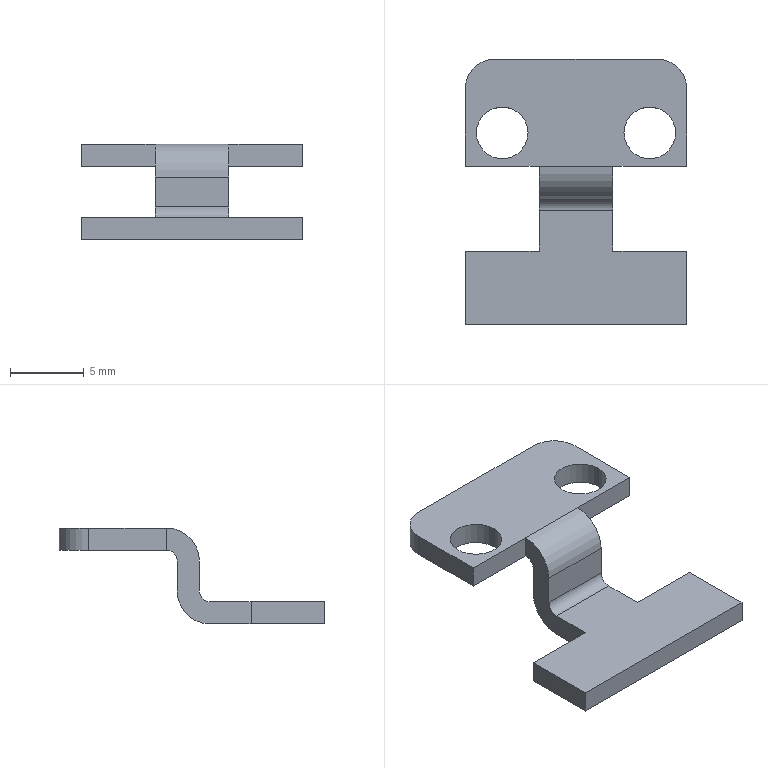Part | STEP file | 02-12 sensor stop plate (Default) | 1 solid | 28 faces | box 15 x 18 x 6.5 mm | volume 315.442 mm3 | plane 18 | cylinder 10 | commonest cylinder face diameters 3.5 x4 1.473 x2 4 x2 4.473 x2
STEP:
#1=CARTESIAN_POINT('',(-6.75,-1.,0.));
#2=VERTEX_POINT('',#1);
#3=CARTESIAN_POINT('',(-3.25,-1.,0.));
#4=VERTEX_POINT('',#3);
#5=CARTESIAN_POINT('',(-5.,-1.,0.));
#6=DIRECTION('',(0.,0.,1.));
#7=DIRECTION('',(1.,0.,0.));
#8=AXIS2_PLACEMENT_3D('',#5,#6,#7);
#9=CIRCLE('',#8,1.75);
#10=EDGE_CURVE('',#2,#4,#9,.T.);
#11=ORIENTED_EDGE('',*,*,#10,.T.);
#12=CARTESIAN_POINT('',(-3.25,-1.,-1.5));
#13=VERTEX_POINT('',#12);
#14=CARTESIAN_POINT('',(-3.25,-1.,11.5));
#15=DIRECTION('',(0.,0.,-1.));
#16=VECTOR('',#15,1000.);
#17=LINE('',#14,#16);
#18=EDGE_CURVE('',#4,#13,#17,.T.);
#19=ORIENTED_EDGE('',*,*,#18,.T.);
#20=CARTESIAN_POINT('',(-6.75,-1.,-1.5));
#21=VERTEX_POINT('',#20);
#22=CARTESIAN_POINT('',(-5.,-1.,-1.5));
#23=DIRECTION('',(0.,0.,-1.));
#24=DIRECTION('',(-1.,0.,0.));
#25=AXIS2_PLACEMENT_3D('',#22,#23,#24);
#26=CIRCLE('',#25,1.75);
#27=EDGE_CURVE('',#13,#21,#26,.T.);
#28=ORIENTED_EDGE('',*,*,#27,.T.);
#29=CARTESIAN_POINT('',(-6.75,-1.,11.5));
#30=DIRECTION('',(0.,0.,-1.));
#31=VECTOR('',#30,1000.);
#32=LINE('',#29,#31);
#33=EDGE_CURVE('',#2,#21,#32,.T.);
#34=ORIENTED_EDGE('',*,*,#33,.F.);
#35=EDGE_LOOP('',(#11,#19,#28,#34));
#36=FACE_OUTER_BOUND('',#35,.T.);
#37=CARTESIAN_POINT('',(-5.,-1.,11.5));
#38=DIRECTION('',(0.,0.,-1.));
#39=DIRECTION('',(-1.,0.,0.));
#40=AXIS2_PLACEMENT_3D('',#37,#38,#39);
#41=CYLINDRICAL_SURFACE('',#40,1.75);
#42=ADVANCED_FACE('',(#36),#41,.F.);
#43=CARTESIAN_POINT('',(3.25,-1.,0.));
#44=VERTEX_POINT('',#43);
#45=CARTESIAN_POINT('',(6.75,-1.,0.));
#46=VERTEX_POINT('',#45);
#47=CARTESIAN_POINT('',(5.,-1.,0.));
#48=DIRECTION('',(0.,0.,1.));
#49=DIRECTION('',(1.,0.,0.));
#50=AXIS2_PLACEMENT_3D('',#47,#48,#49);
#51=CIRCLE('',#50,1.75);
#52=EDGE_CURVE('',#44,#46,#51,.T.);
#53=ORIENTED_EDGE('',*,*,#52,.T.);
#54=CARTESIAN_POINT('',(6.75,-1.,-1.5));
#55=VERTEX_POINT('',#54);
#56=CARTESIAN_POINT('',(6.75,-1.,11.5));
#57=DIRECTION('',(0.,0.,-1.));
#58=VECTOR('',#57,1000.);
#59=LINE('',#56,#58);
#60=EDGE_CURVE('',#46,#55,#59,.T.);
#61=ORIENTED_EDGE('',*,*,#60,.T.);
#62=CARTESIAN_POINT('',(3.25,-1.,-1.5));
#63=VERTEX_POINT('',#62);
#64=CARTESIAN_POINT('',(5.,-1.,-1.5));
#65=DIRECTION('',(0.,0.,-1.));
#66=DIRECTION('',(-1.,0.,0.));
#67=AXIS2_PLACEMENT_3D('',#64,#65,#66);
#68=CIRCLE('',#67,1.75);
#69=EDGE_CURVE('',#55,#63,#68,.T.);
#70=ORIENTED_EDGE('',*,*,#69,.T.);
#71=CARTESIAN_POINT('',(3.25,-1.,11.5));
#72=DIRECTION('',(0.,0.,-1.));
#73=VECTOR('',#72,1000.);
#74=LINE('',#71,#73);
#75=EDGE_CURVE('',#44,#63,#74,.T.);
#76=ORIENTED_EDGE('',*,*,#75,.F.);
#77=EDGE_LOOP('',(#53,#61,#70,#76));
#78=FACE_OUTER_BOUND('',#77,.T.);
#79=CARTESIAN_POINT('',(5.,-1.,11.5));
#80=DIRECTION('',(0.,0.,-1.));
#81=DIRECTION('',(-1.,0.,0.));
#82=AXIS2_PLACEMENT_3D('',#79,#80,#81);
#83=CYLINDRICAL_SURFACE('',#82,1.75);
#84=ADVANCED_FACE('',(#78),#83,.F.);
#85=CARTESIAN_POINT('',(2.5,-5.5,-4.263));
#86=VERTEX_POINT('',#85);
#87=CARTESIAN_POINT('',(-2.5,-5.5,-4.263));
#88=VERTEX_POINT('',#87);
#89=CARTESIAN_POINT('',(7.5,-5.5,-4.263));
#90=DIRECTION('',(-1.,0.,0.));
#91=VECTOR('',#90,1000.);
#92=LINE('',#89,#91);
#93=EDGE_CURVE('',#86,#88,#92,.T.);
#94=ORIENTED_EDGE('',*,*,#93,.F.);
#95=CARTESIAN_POINT('',(2.5,-5.5,-2.237));
#96=VERTEX_POINT('',#95);
#97=CARTESIAN_POINT('',(2.5,-5.5,-1.5));
#98=DIRECTION('',(0.,0.,1.));
#99=VECTOR('',#98,1000.);
#100=LINE('',#97,#99);
#101=EDGE_CURVE('',#86,#96,#100,.T.);
#102=ORIENTED_EDGE('',*,*,#101,.T.);
#103=CARTESIAN_POINT('',(-2.5,-5.5,-2.237));
#104=VERTEX_POINT('',#103);
#105=CARTESIAN_POINT('',(-7.5,-5.5,-2.237));
#106=DIRECTION('',(1.,0.,0.));
#107=VECTOR('',#106,1000.);
#108=LINE('',#105,#107);
#109=EDGE_CURVE('',#104,#96,#108,.T.);
#110=ORIENTED_EDGE('',*,*,#109,.F.);
#111=CARTESIAN_POINT('',(-2.5,-5.5,-1.5));
#112=DIRECTION('',(0.,0.,-1.));
#113=VECTOR('',#112,1000.);
#114=LINE('',#111,#113);
#115=EDGE_CURVE('',#104,#88,#114,.T.);
#116=ORIENTED_EDGE('',*,*,#115,.T.);
#117=EDGE_LOOP('',(#94,#102,#110,#116));
#118=FACE_OUTER_BOUND('',#117,.T.);
#119=CARTESIAN_POINT('',(-7.5,-5.5,-1.5));
#120=DIRECTION('',(0.,1.,0.));
#121=DIRECTION('',(0.,0.,1.));
#122=AXIS2_PLACEMENT_3D('',#119,#120,#121);
#123=PLANE('',#122);
#124=ADVANCED_FACE('',(#118),#123,.F.);
#125=CARTESIAN_POINT('',(2.5,-4.,-4.263));
#126=VERTEX_POINT('',#125);
#127=CARTESIAN_POINT('',(2.5,-4.,-2.237));
#128=VERTEX_POINT('',#127);
#129=CARTESIAN_POINT('',(2.5,-4.,-1.5));
#130=DIRECTION('',(0.,0.,1.));
#131=VECTOR('',#130,1000.);
#132=LINE('',#129,#131);
#133=EDGE_CURVE('',#126,#128,#132,.T.);
#134=ORIENTED_EDGE('',*,*,#133,.F.);
#135=CARTESIAN_POINT('',(-2.5,-4.,-4.263));
#136=VERTEX_POINT('',#135);
#137=CARTESIAN_POINT('',(7.5,-4.,-4.263));
#138=DIRECTION('',(-1.,0.,0.));
#139=VECTOR('',#138,1000.);
#140=LINE('',#137,#139);
#141=EDGE_CURVE('',#126,#136,#140,.T.);
#142=ORIENTED_EDGE('',*,*,#141,.T.);
#143=CARTESIAN_POINT('',(-2.5,-4.,-2.237));
#144=VERTEX_POINT('',#143);
#145=CARTESIAN_POINT('',(-2.5,-4.,-1.5));
#146=DIRECTION('',(0.,0.,-1.));
#147=VECTOR('',#146,1000.);
#148=LINE('',#145,#147);
#149=EDGE_CURVE('',#144,#136,#148,.T.);
#150=ORIENTED_EDGE('',*,*,#149,.F.);
#151=CARTESIAN_POINT('',(7.5,-4.,-2.237));
#152=DIRECTION('',(-1.,0.,0.));
#153=VECTOR('',#152,1000.);
#154=LINE('',#151,#153);
#155=EDGE_CURVE('',#128,#144,#154,.T.);
#156=ORIENTED_EDGE('',*,*,#155,.F.);
#157=EDGE_LOOP('',(#134,#142,#150,#156));
#158=FACE_OUTER_BOUND('',#157,.T.);
#159=CARTESIAN_POINT('',(-7.5,-4.,-1.5));
#160=DIRECTION('',(0.,1.,0.));
#161=DIRECTION('',(0.,0.,1.));
#162=AXIS2_PLACEMENT_3D('',#159,#160,#161);
#163=PLANE('',#162);
#164=ADVANCED_FACE('',(#158),#163,.T.);
#165=CARTESIAN_POINT('',(-7.5,2.,0.));
#166=VERTEX_POINT('',#165);
#167=CARTESIAN_POINT('',(-7.5,-3.263,0.));
#168=VERTEX_POINT('',#167);
#169=CARTESIAN_POINT('',(-7.5,4.,0.));
#170=DIRECTION('',(0.,-1.,0.));
#171=VECTOR('',#170,1000.);
#172=LINE('',#169,#171);
#173=EDGE_CURVE('',#166,#168,#172,.T.);
#174=ORIENTED_EDGE('',*,*,#173,.F.);
#175=CARTESIAN_POINT('',(-7.5,2.,-1.5));
#176=VERTEX_POINT('',#175);
#177=CARTESIAN_POINT('',(-7.5,2.,-1.5));
#178=DIRECTION('',(0.,0.,-1.));
#179=VECTOR('',#178,1000.);
#180=LINE('',#177,#179);
#181=EDGE_CURVE('',#166,#176,#180,.T.);
#182=ORIENTED_EDGE('',*,*,#181,.T.);
#183=CARTESIAN_POINT('',(-7.5,-3.263,-1.5));
#184=VERTEX_POINT('',#183);
#185=CARTESIAN_POINT('',(-7.5,4.,-1.5));
#186=DIRECTION('',(0.,-1.,0.));
#187=VECTOR('',#186,1000.);
#188=LINE('',#185,#187);
#189=EDGE_CURVE('',#176,#184,#188,.T.);
#190=ORIENTED_EDGE('',*,*,#189,.T.);
#191=CARTESIAN_POINT('',(-7.5,-3.263,-1.5));
#192=DIRECTION('',(0.,0.,1.));
#193=VECTOR('',#192,1000.);
#194=LINE('',#191,#193);
#195=EDGE_CURVE('',#184,#168,#194,.T.);
#196=ORIENTED_EDGE('',*,*,#195,.T.);
#197=EDGE_LOOP('',(#174,#182,#190,#196));
#198=FACE_OUTER_BOUND('',#197,.T.);
#199=CARTESIAN_POINT('',(-7.5,4.,-1.5));
#200=DIRECTION('',(-1.,0.,0.));
#201=DIRECTION('',(0.,-1.,0.));
#202=AXIS2_PLACEMENT_3D('',#199,#200,#201);
#203=PLANE('',#202);
#204=ADVANCED_FACE('',(#198),#203,.T.);
#205=CARTESIAN_POINT('',(-5.,-1.,-1.5));
#206=DIRECTION('',(0.,0.,-1.));
#207=DIRECTION('',(-1.,0.,0.));
#208=AXIS2_PLACEMENT_3D('',#205,#206,#207);
#209=CIRCLE('',#208,1.75);
#210=EDGE_CURVE('',#21,#13,#209,.T.);
#211=ORIENTED_EDGE('',*,*,#210,.F.);
#212=ORIENTED_EDGE('',*,*,#27,.F.);
#213=EDGE_LOOP('',(#211,#212));
#214=FACE_BOUND('',#213,.T.);
#215=CARTESIAN_POINT('',(5.,-1.,-1.5));
#216=DIRECTION('',(0.,0.,-1.));
#217=DIRECTION('',(-1.,0.,0.));
#218=AXIS2_PLACEMENT_3D('',#215,#216,#217);
#219=CIRCLE('',#218,1.75);
#220=EDGE_CURVE('',#63,#55,#219,.T.);
#221=ORIENTED_EDGE('',*,*,#220,.F.);
#222=ORIENTED_EDGE('',*,*,#69,.F.);
#223=EDGE_LOOP('',(#221,#222));
#224=FACE_BOUND('',#223,.T.);
#225=ORIENTED_EDGE('',*,*,#189,.F.);
#226=CARTESIAN_POINT('',(-5.5,4.,-1.5));
#227=VERTEX_POINT('',#226);
#228=CARTESIAN_POINT('',(-5.5,2.,-1.5));
#229=DIRECTION('',(0.,0.,-1.));
#230=DIRECTION('',(1.,0.,0.));
#231=AXIS2_PLACEMENT_3D('',#228,#229,#230);
#232=CIRCLE('',#231,2.);
#233=EDGE_CURVE('',#176,#227,#232,.T.);
#234=ORIENTED_EDGE('',*,*,#233,.T.);
#235=CARTESIAN_POINT('',(5.5,4.,-1.5));
#236=VERTEX_POINT('',#235);
#237=CARTESIAN_POINT('',(-7.5,4.,-1.5));
#238=DIRECTION('',(-1.,0.,0.));
#239=VECTOR('',#238,1000.);
#240=LINE('',#237,#239);
#241=EDGE_CURVE('',#236,#227,#240,.T.);
#242=ORIENTED_EDGE('',*,*,#241,.F.);
#243=CARTESIAN_POINT('',(7.5,2.,-1.5));
#244=VERTEX_POINT('',#243);
#245=CARTESIAN_POINT('',(5.5,2.,-1.5));
#246=DIRECTION('',(0.,0.,-1.));
#247=DIRECTION('',(1.,0.,0.));
#248=AXIS2_PLACEMENT_3D('',#245,#246,#247);
#249=CIRCLE('',#248,2.);
#250=EDGE_CURVE('',#236,#244,#249,.T.);
#251=ORIENTED_EDGE('',*,*,#250,.T.);
#252=CARTESIAN_POINT('',(7.5,-3.263,-1.5));
#253=VERTEX_POINT('',#252);
#254=CARTESIAN_POINT('',(7.5,4.,-1.5));
#255=DIRECTION('',(0.,1.,0.));
#256=VECTOR('',#255,1000.);
#257=LINE('',#254,#256);
#258=EDGE_CURVE('',#253,#244,#257,.T.);
#259=ORIENTED_EDGE('',*,*,#258,.F.);
#260=CARTESIAN_POINT('',(2.5,-3.263,-1.5));
#261=VERTEX_POINT('',#260);
#262=CARTESIAN_POINT('',(-7.5,-3.263,-1.5));
#263=DIRECTION('',(1.,0.,0.));
#264=VECTOR('',#263,1000.);
#265=LINE('',#262,#264);
#266=EDGE_CURVE('',#261,#253,#265,.T.);
#267=ORIENTED_EDGE('',*,*,#266,.F.);
#268=CARTESIAN_POINT('',(-2.5,-3.263,-1.5));
#269=VERTEX_POINT('',#268);
#270=CARTESIAN_POINT('',(-7.5,-3.263,-1.5));
#271=DIRECTION('',(1.,0.,0.));
#272=VECTOR('',#271,1000.);
#273=LINE('',#270,#272);
#274=EDGE_CURVE('',#269,#261,#273,.T.);
#275=ORIENTED_EDGE('',*,*,#274,.F.);
#276=CARTESIAN_POINT('',(-7.5,-3.263,-1.5));
#277=DIRECTION('',(1.,0.,0.));
#278=VECTOR('',#277,1000.);
#279=LINE('',#276,#278);
#280=EDGE_CURVE('',#184,#269,#279,.T.);
#281=ORIENTED_EDGE('',*,*,#280,.F.);
#282=EDGE_LOOP('',(#225,#234,#242,#251,#259,#267,#275,#281));
#283=FACE_OUTER_BOUND('',#282,.T.);
#284=CARTESIAN_POINT('',(7.5,-4.,-1.5));
#285=DIRECTION('',(0.,0.,1.));
#286=DIRECTION('',(1.,0.,0.));
#287=AXIS2_PLACEMENT_3D('',#284,#285,#286);
#288=PLANE('',#287);
#289=ADVANCED_FACE('',(#214,#224,#283),#288,.F.);
#290=ORIENTED_EDGE('',*,*,#10,.F.);
#291=CARTESIAN_POINT('',(-5.,-1.,0.));
#292=DIRECTION('',(0.,0.,1.));
#293=DIRECTION('',(1.,0.,0.));
#294=AXIS2_PLACEMENT_3D('',#291,#292,#293);
#295=CIRCLE('',#294,1.75);
#296=EDGE_CURVE('',#4,#2,#295,.T.);
#297=ORIENTED_EDGE('',*,*,#296,.F.);
#298=EDGE_LOOP('',(#290,#297));
#299=FACE_BOUND('',#298,.T.);
#300=ORIENTED_EDGE('',*,*,#52,.F.);
#301=CARTESIAN_POINT('',(5.,-1.,0.));
#302=DIRECTION('',(0.,0.,1.));
#303=DIRECTION('',(1.,0.,0.));
#304=AXIS2_PLACEMENT_3D('',#301,#302,#303);
#305=CIRCLE('',#304,1.75);
#306=EDGE_CURVE('',#46,#44,#305,.T.);
#307=ORIENTED_EDGE('',*,*,#306,.F.);
#308=EDGE_LOOP('',(#300,#307));
#309=FACE_BOUND('',#308,.T.);
#310=CARTESIAN_POINT('',(5.5,4.,0.));
#311=VERTEX_POINT('',#310);
#312=CARTESIAN_POINT('',(-5.5,4.,0.));
#313=VERTEX_POINT('',#312);
#314=CARTESIAN_POINT('',(-7.5,4.,0.));
#315=DIRECTION('',(-1.,0.,0.));
#316=VECTOR('',#315,1000.);
#317=LINE('',#314,#316);
#318=EDGE_CURVE('',#311,#313,#317,.T.);
#319=ORIENTED_EDGE('',*,*,#318,.T.);
#320=CARTESIAN_POINT('',(-5.5,2.,0.));
#321=DIRECTION('',(0.,0.,1.));
#322=DIRECTION('',(1.,0.,0.));
#323=AXIS2_PLACEMENT_3D('',#320,#321,#322);
#324=CIRCLE('',#323,2.);
#325=EDGE_CURVE('',#313,#166,#324,.T.);
#326=ORIENTED_EDGE('',*,*,#325,.T.);
#327=ORIENTED_EDGE('',*,*,#173,.T.);
#328=CARTESIAN_POINT('',(-2.5,-3.263,0.));
#329=VERTEX_POINT('',#328);
#330=CARTESIAN_POINT('',(-7.5,-3.263,0.));
#331=DIRECTION('',(1.,0.,0.));
#332=VECTOR('',#331,1000.);
#333=LINE('',#330,#332);
#334=EDGE_CURVE('',#168,#329,#333,.T.);
#335=ORIENTED_EDGE('',*,*,#334,.T.);
#336=CARTESIAN_POINT('',(2.5,-3.263,0.));
#337=VERTEX_POINT('',#336);
#338=CARTESIAN_POINT('',(-7.5,-3.263,0.));
#339=DIRECTION('',(1.,0.,0.));
#340=VECTOR('',#339,1000.);
#341=LINE('',#338,#340);
#342=EDGE_CURVE('',#329,#337,#341,.T.);
#343=ORIENTED_EDGE('',*,*,#342,.T.);
#344=CARTESIAN_POINT('',(7.5,-3.263,0.));
#345=VERTEX_POINT('',#344);
#346=CARTESIAN_POINT('',(7.5,-3.263,0.));
#347=DIRECTION('',(1.,0.,0.));
#348=VECTOR('',#347,1000.);
#349=LINE('',#346,#348);
#350=EDGE_CURVE('',#337,#345,#349,.T.);
#351=ORIENTED_EDGE('',*,*,#350,.T.);
#352=CARTESIAN_POINT('',(7.5,2.,0.));
#353=VERTEX_POINT('',#352);
#354=CARTESIAN_POINT('',(7.5,4.,0.));
#355=DIRECTION('',(0.,1.,0.));
#356=VECTOR('',#355,1000.);
#357=LINE('',#354,#356);
#358=EDGE_CURVE('',#345,#353,#357,.T.);
#359=ORIENTED_EDGE('',*,*,#358,.T.);
#360=CARTESIAN_POINT('',(5.5,2.,0.));
#361=DIRECTION('',(0.,0.,1.));
#362=DIRECTION('',(1.,0.,0.));
#363=AXIS2_PLACEMENT_3D('',#360,#361,#362);
#364=CIRCLE('',#363,2.);
#365=EDGE_CURVE('',#353,#311,#364,.T.);
#366=ORIENTED_EDGE('',*,*,#365,.T.);
#367=EDGE_LOOP('',(#319,#326,#327,#335,#343,#351,#359,#366));
#368=FACE_OUTER_BOUND('',#367,.T.);
#369=CARTESIAN_POINT('',(7.5,-4.,0.));
#370=DIRECTION('',(0.,0.,1.));
#371=DIRECTION('',(1.,0.,0.));
#372=AXIS2_PLACEMENT_3D('',#369,#370,#371);
#373=PLANE('',#372);
#374=ADVANCED_FACE('',(#299,#309,#368),#373,.T.);
#375=ORIENTED_EDGE('',*,*,#258,.T.);
#376=CARTESIAN_POINT('',(7.5,2.,-1.5));
#377=DIRECTION('',(0.,0.,1.));
#378=VECTOR('',#377,1000.);
#379=LINE('',#376,#378);
#380=EDGE_CURVE('',#244,#353,#379,.T.);
#381=ORIENTED_EDGE('',*,*,#380,.T.);
#382=ORIENTED_EDGE('',*,*,#358,.F.);
#383=CARTESIAN_POINT('',(7.5,-3.263,-1.5));
#384=DIRECTION('',(0.,0.,1.));
#385=VECTOR('',#384,1000.);
#386=LINE('',#383,#385);
#387=EDGE_CURVE('',#253,#345,#386,.T.);
#388=ORIENTED_EDGE('',*,*,#387,.F.);
#389=EDGE_LOOP('',(#375,#381,#382,#388));
#390=FACE_OUTER_BOUND('',#389,.T.);
#391=CARTESIAN_POINT('',(7.5,4.,-1.5));
#392=DIRECTION('',(1.,0.,0.));
#393=DIRECTION('',(0.,1.,0.));
#394=AXIS2_PLACEMENT_3D('',#391,#392,#393);
#395=PLANE('',#394);
#396=ADVANCED_FACE('',(#390),#395,.T.);
#397=ORIENTED_EDGE('',*,*,#241,.T.);
#398=CARTESIAN_POINT('',(-5.5,4.,-1.5));
#399=DIRECTION('',(0.,0.,1.));
#400=VECTOR('',#399,1000.);
#401=LINE('',#398,#400);
#402=EDGE_CURVE('',#227,#313,#401,.T.);
#403=ORIENTED_EDGE('',*,*,#402,.T.);
#404=ORIENTED_EDGE('',*,*,#318,.F.);
#405=CARTESIAN_POINT('',(5.5,4.,-1.5));
#406=DIRECTION('',(0.,0.,-1.));
#407=VECTOR('',#406,1000.);
#408=LINE('',#405,#407);
#409=EDGE_CURVE('',#311,#236,#408,.T.);
#410=ORIENTED_EDGE('',*,*,#409,.T.);
#411=EDGE_LOOP('',(#397,#403,#404,#410));
#412=FACE_OUTER_BOUND('',#411,.T.);
#413=CARTESIAN_POINT('',(-7.5,4.,-1.5));
#414=DIRECTION('',(0.,1.,0.));
#415=DIRECTION('',(0.,0.,1.));
#416=AXIS2_PLACEMENT_3D('',#413,#414,#415);
#417=PLANE('',#416);
#418=ADVANCED_FACE('',(#412),#417,.T.);
#419=CARTESIAN_POINT('',(2.5,-3.263,-2.237));
#420=DIRECTION('',(1.,0.,0.));
#421=DIRECTION('',(0.,-1.,0.));
#422=AXIS2_PLACEMENT_3D('',#419,#420,#421);
#423=CIRCLE('',#422,2.237);
#424=EDGE_CURVE('',#337,#96,#423,.T.);
#425=ORIENTED_EDGE('',*,*,#424,.F.);
#426=ORIENTED_EDGE('',*,*,#342,.F.);
#427=CARTESIAN_POINT('',(-2.5,-3.263,-2.237));
#428=DIRECTION('',(-1.,0.,0.));
#429=DIRECTION('',(0.,1.,0.));
#430=AXIS2_PLACEMENT_3D('',#427,#428,#429);
#431=CIRCLE('',#430,2.237);
#432=EDGE_CURVE('',#104,#329,#431,.T.);
#433=ORIENTED_EDGE('',*,*,#432,.F.);
#434=ORIENTED_EDGE('',*,*,#109,.T.);
#435=EDGE_LOOP('',(#425,#426,#433,#434));
#436=FACE_OUTER_BOUND('',#435,.T.);
#437=CARTESIAN_POINT('',(-7.5,-3.263,-2.237));
#438=DIRECTION('',(-1.,0.,0.));
#439=DIRECTION('',(0.,-1.,0.));
#440=AXIS2_PLACEMENT_3D('',#437,#438,#439);
#441=CYLINDRICAL_SURFACE('',#440,2.237);
#442=ADVANCED_FACE('',(#436),#441,.T.);
#443=ORIENTED_EDGE('',*,*,#274,.T.);
#444=CARTESIAN_POINT('',(2.5,-3.263,-2.237));
#445=DIRECTION('',(1.,0.,0.));
#446=DIRECTION('',(0.,-1.,0.));
#447=AXIS2_PLACEMENT_3D('',#444,#445,#446);
#448=CIRCLE('',#447,0.7366);
#449=EDGE_CURVE('',#261,#128,#448,.T.);
#450=ORIENTED_EDGE('',*,*,#449,.T.);
#451=ORIENTED_EDGE('',*,*,#155,.T.);
#452=CARTESIAN_POINT('',(-2.5,-3.263,-2.237));
#453=DIRECTION('',(-1.,0.,0.));
#454=DIRECTION('',(0.,1.,0.));
#455=AXIS2_PLACEMENT_3D('',#452,#453,#454);
#456=CIRCLE('',#455,0.7366);
#457=EDGE_CURVE('',#144,#269,#456,.T.);
#458=ORIENTED_EDGE('',*,*,#457,.T.);
#459=EDGE_LOOP('',(#443,#450,#451,#458));
#460=FACE_OUTER_BOUND('',#459,.T.);
#461=CARTESIAN_POINT('',(-7.5,-3.263,-2.237));
#462=DIRECTION('',(-1.,0.,0.));
#463=DIRECTION('',(0.,-1.,0.));
#464=AXIS2_PLACEMENT_3D('',#461,#462,#463);
#465=CYLINDRICAL_SURFACE('',#464,0.7366);
#466=ADVANCED_FACE('',(#460),#465,.F.);
#467=CARTESIAN_POINT('',(2.5,-6.237,-6.5));
#468=VERTEX_POINT('',#467);
#469=CARTESIAN_POINT('',(2.5,-6.237,-4.263));
#470=DIRECTION('',(1.,0.,0.));
#471=DIRECTION('',(0.,-1.,0.));
#472=AXIS2_PLACEMENT_3D('',#469,#470,#471);
#473=CIRCLE('',#472,2.237);
#474=EDGE_CURVE('',#468,#126,#473,.T.);
#475=ORIENTED_EDGE('',*,*,#474,.F.);
#476=CARTESIAN_POINT('',(-2.5,-6.237,-6.5));
#477=VERTEX_POINT('',#476);
#478=CARTESIAN_POINT('',(7.5,-6.237,-6.5));
#479=DIRECTION('',(1.,0.,0.));
#480=VECTOR('',#479,1000.);
#481=LINE('',#478,#480);
#482=EDGE_CURVE('',#477,#468,#481,.T.);
#483=ORIENTED_EDGE('',*,*,#482,.F.);
#484=CARTESIAN_POINT('',(-2.5,-6.237,-4.263));
#485=DIRECTION('',(-1.,0.,0.));
#486=DIRECTION('',(0.,1.,0.));
#487=AXIS2_PLACEMENT_3D('',#484,#485,#486);
#488=CIRCLE('',#487,2.237);
#489=EDGE_CURVE('',#136,#477,#488,.T.);
#490=ORIENTED_EDGE('',*,*,#489,.F.);
#491=ORIENTED_EDGE('',*,*,#141,.F.);
#492=EDGE_LOOP('',(#475,#483,#490,#491));
#493=FACE_OUTER_BOUND('',#492,.T.);
#494=CARTESIAN_POINT('',(7.5,-6.237,-4.263));
#495=DIRECTION('',(1.,0.,0.));
#496=DIRECTION('',(0.,0.,-1.));
#497=AXIS2_PLACEMENT_3D('',#494,#495,#496);
#498=CYLINDRICAL_SURFACE('',#497,2.237);
#499=ADVANCED_FACE('',(#493),#498,.T.);
#500=CARTESIAN_POINT('',(-2.5,-6.237,-5.));
#501=VERTEX_POINT('',#500);
#502=CARTESIAN_POINT('',(2.5,-6.237,-5.));
#503=VERTEX_POINT('',#502);
#504=CARTESIAN_POINT('',(-7.5,-6.237,-5.));
#505=DIRECTION('',(1.,0.,0.));
#506=VECTOR('',#505,1000.);
#507=LINE('',#504,#506);
#508=EDGE_CURVE('',#501,#503,#507,.T.);
#509=ORIENTED_EDGE('',*,*,#508,.T.);
#510=CARTESIAN_POINT('',(2.5,-6.237,-4.263));
#511=DIRECTION('',(1.,0.,0.));
#512=DIRECTION('',(0.,-1.,0.));
#513=AXIS2_PLACEMENT_3D('',#510,#511,#512);
#514=CIRCLE('',#513,0.7366);
#515=EDGE_CURVE('',#503,#86,#514,.T.);
#516=ORIENTED_EDGE('',*,*,#515,.T.);
#517=ORIENTED_EDGE('',*,*,#93,.T.);
#518=CARTESIAN_POINT('',(-2.5,-6.237,-4.263));
#519=DIRECTION('',(-1.,0.,0.));
#520=DIRECTION('',(0.,1.,0.));
#521=AXIS2_PLACEMENT_3D('',#518,#519,#520);
#522=CIRCLE('',#521,0.7366);
#523=EDGE_CURVE('',#88,#501,#522,.T.);
#524=ORIENTED_EDGE('',*,*,#523,.T.);
#525=EDGE_LOOP('',(#509,#516,#517,#524));
#526=FACE_OUTER_BOUND('',#525,.T.);
#527=CARTESIAN_POINT('',(7.5,-6.237,-4.263));
#528=DIRECTION('',(1.,0.,0.));
#529=DIRECTION('',(0.,0.,-1.));
#530=AXIS2_PLACEMENT_3D('',#527,#528,#529);
#531=CYLINDRICAL_SURFACE('',#530,0.7366);
#532=ADVANCED_FACE('',(#526),#531,.F.);
#533=CARTESIAN_POINT('',(2.5,-9.,-6.5));
#534=VERTEX_POINT('',#533);
#535=CARTESIAN_POINT('',(2.5,-3.263,-6.5));
#536=DIRECTION('',(0.,1.,0.));
#537=VECTOR('',#536,1000.);
#538=LINE('',#535,#537);
#539=EDGE_CURVE('',#534,#468,#538,.T.);
#540=ORIENTED_EDGE('',*,*,#539,.F.);
#541=CARTESIAN_POINT('',(7.5,-9.,-6.5));
#542=VERTEX_POINT('',#541);
#543=CARTESIAN_POINT('',(7.5,-9.,-6.5));
#544=DIRECTION('',(1.,0.,0.));
#545=VECTOR('',#544,1000.);
#546=LINE('',#543,#545);
#547=EDGE_CURVE('',#534,#542,#546,.T.);
#548=ORIENTED_EDGE('',*,*,#547,.T.);
#549=CARTESIAN_POINT('',(7.5,-14.,-6.5));
#550=VERTEX_POINT('',#549);
#551=CARTESIAN_POINT('',(7.5,-9.,-6.5));
#552=DIRECTION('',(0.,-1.,0.));
#553=VECTOR('',#552,1000.);
#554=LINE('',#551,#553);
#555=EDGE_CURVE('',#542,#550,#554,.T.);
#556=ORIENTED_EDGE('',*,*,#555,.T.);
#557=CARTESIAN_POINT('',(-7.5,-14.,-6.5));
#558=VERTEX_POINT('',#557);
#559=CARTESIAN_POINT('',(7.5,-14.,-6.5));
#560=DIRECTION('',(1.,0.,0.));
#561=VECTOR('',#560,1000.);
#562=LINE('',#559,#561);
#563=EDGE_CURVE('',#558,#550,#562,.T.);
#564=ORIENTED_EDGE('',*,*,#563,.F.);
#565=CARTESIAN_POINT('',(-7.5,-9.,-6.5));
#566=VERTEX_POINT('',#565);
#567=CARTESIAN_POINT('',(-7.5,-9.,-6.5));
#568=DIRECTION('',(0.,1.,0.));
#569=VECTOR('',#568,1000.);
#570=LINE('',#567,#569);
#571=EDGE_CURVE('',#558,#566,#570,.T.);
#572=ORIENTED_EDGE('',*,*,#571,.T.);
#573=CARTESIAN_POINT('',(-2.5,-9.,-6.5));
#574=VERTEX_POINT('',#573);
#575=CARTESIAN_POINT('',(7.5,-9.,-6.5));
#576=DIRECTION('',(1.,0.,0.));
#577=VECTOR('',#576,1000.);
#578=LINE('',#575,#577);
#579=EDGE_CURVE('',#566,#574,#578,.T.);
#580=ORIENTED_EDGE('',*,*,#579,.T.);
#581=CARTESIAN_POINT('',(-2.5,-3.263,-6.5));
#582=DIRECTION('',(0.,-1.,0.));
#583=VECTOR('',#582,1000.);
#584=LINE('',#581,#583);
#585=EDGE_CURVE('',#477,#574,#584,.T.);
#586=ORIENTED_EDGE('',*,*,#585,.F.);
#587=ORIENTED_EDGE('',*,*,#482,.T.);
#588=EDGE_LOOP('',(#540,#548,#556,#564,#572,#580,#586,#587));
#589=FACE_OUTER_BOUND('',#588,.T.);
#590=CARTESIAN_POINT('',(7.5,-5.5,-6.5));
#591=DIRECTION('',(0.,0.,-1.));
#592=DIRECTION('',(-1.,0.,0.));
#593=AXIS2_PLACEMENT_3D('',#590,#591,#592);
#594=PLANE('',#593);
#595=ADVANCED_FACE('',(#589),#594,.T.);
#596=CARTESIAN_POINT('',(-2.5,-9.,-5.));
#597=VERTEX_POINT('',#596);
#598=CARTESIAN_POINT('',(-2.5,-5.5,-5.));
#599=DIRECTION('',(0.,-1.,0.));
#600=VECTOR('',#599,1000.);
#601=LINE('',#598,#600);
#602=EDGE_CURVE('',#501,#597,#601,.T.);
#603=ORIENTED_EDGE('',*,*,#602,.T.);
#604=CARTESIAN_POINT('',(-7.5,-9.,-5.));
#605=VERTEX_POINT('',#604);
#606=CARTESIAN_POINT('',(7.5,-9.,-5.));
#607=DIRECTION('',(1.,0.,0.));
#608=VECTOR('',#607,1000.);
#609=LINE('',#606,#608);
#610=EDGE_CURVE('',#605,#597,#609,.T.);
#611=ORIENTED_EDGE('',*,*,#610,.F.);
#612=CARTESIAN_POINT('',(-7.5,-14.,-5.));
#613=VERTEX_POINT('',#612);
#614=CARTESIAN_POINT('',(-7.5,-9.,-5.));
#615=DIRECTION('',(0.,1.,0.));
#616=VECTOR('',#615,1000.);
#617=LINE('',#614,#616);
#618=EDGE_CURVE('',#613,#605,#617,.T.);
#619=ORIENTED_EDGE('',*,*,#618,.F.);
#620=CARTESIAN_POINT('',(7.5,-14.,-5.));
#621=VERTEX_POINT('',#620);
#622=CARTESIAN_POINT('',(7.5,-14.,-5.));
#623=DIRECTION('',(1.,0.,0.));
#624=VECTOR('',#623,1000.);
#625=LINE('',#622,#624);
#626=EDGE_CURVE('',#613,#621,#625,.T.);
#627=ORIENTED_EDGE('',*,*,#626,.T.);
#628=CARTESIAN_POINT('',(7.5,-9.,-5.));
#629=VERTEX_POINT('',#628);
#630=CARTESIAN_POINT('',(7.5,-9.,-5.));
#631=DIRECTION('',(0.,-1.,0.));
#632=VECTOR('',#631,1000.);
#633=LINE('',#630,#632);
#634=EDGE_CURVE('',#629,#621,#633,.T.);
#635=ORIENTED_EDGE('',*,*,#634,.F.);
#636=CARTESIAN_POINT('',(2.5,-9.,-5.));
#637=VERTEX_POINT('',#636);
#638=CARTESIAN_POINT('',(7.5,-9.,-5.));
#639=DIRECTION('',(1.,0.,0.));
#640=VECTOR('',#639,1000.);
#641=LINE('',#638,#640);
#642=EDGE_CURVE('',#637,#629,#641,.T.);
#643=ORIENTED_EDGE('',*,*,#642,.F.);
#644=CARTESIAN_POINT('',(2.5,-5.5,-5.));
#645=DIRECTION('',(0.,1.,0.));
#646=VECTOR('',#645,1000.);
#647=LINE('',#644,#646);
#648=EDGE_CURVE('',#637,#503,#647,.T.);
#649=ORIENTED_EDGE('',*,*,#648,.T.);
#650=ORIENTED_EDGE('',*,*,#508,.F.);
#651=EDGE_LOOP('',(#603,#611,#619,#627,#635,#643,#649,#650));
#652=FACE_OUTER_BOUND('',#651,.T.);
#653=CARTESIAN_POINT('',(7.5,-5.5,-5.));
#654=DIRECTION('',(0.,0.,-1.));
#655=DIRECTION('',(-1.,0.,0.));
#656=AXIS2_PLACEMENT_3D('',#653,#654,#655);
#657=PLANE('',#656);
#658=ADVANCED_FACE('',(#652),#657,.F.);
#659=ORIENTED_EDGE('',*,*,#563,.T.);
#660=CARTESIAN_POINT('',(7.5,-14.,-5.));
#661=DIRECTION('',(0.,0.,-1.));
#662=VECTOR('',#661,1000.);
#663=LINE('',#660,#662);
#664=EDGE_CURVE('',#621,#550,#663,.T.);
#665=ORIENTED_EDGE('',*,*,#664,.F.);
#666=ORIENTED_EDGE('',*,*,#626,.F.);
#667=CARTESIAN_POINT('',(-7.5,-14.,-5.));
#668=DIRECTION('',(0.,0.,-1.));
#669=VECTOR('',#668,1000.);
#670=LINE('',#667,#669);
#671=EDGE_CURVE('',#613,#558,#670,.T.);
#672=ORIENTED_EDGE('',*,*,#671,.T.);
#673=EDGE_LOOP('',(#659,#665,#666,#672));
#674=FACE_OUTER_BOUND('',#673,.T.);
#675=CARTESIAN_POINT('',(7.5,-14.,-6.5));
#676=DIRECTION('',(0.,-1.,0.));
#677=DIRECTION('',(0.,0.,-1.));
#678=AXIS2_PLACEMENT_3D('',#675,#676,#677);
#679=PLANE('',#678);
#680=ADVANCED_FACE('',(#674),#679,.T.);
#681=ORIENTED_EDGE('',*,*,#233,.F.);
#682=ORIENTED_EDGE('',*,*,#181,.F.);
#683=ORIENTED_EDGE('',*,*,#325,.F.);
#684=ORIENTED_EDGE('',*,*,#402,.F.);
#685=EDGE_LOOP('',(#681,#682,#683,#684));
#686=FACE_OUTER_BOUND('',#685,.T.);
#687=CARTESIAN_POINT('',(-5.5,2.,-1.5));
#688=DIRECTION('',(0.,0.,1.));
#689=DIRECTION('',(1.,0.,0.));
#690=AXIS2_PLACEMENT_3D('',#687,#688,#689);
#691=CYLINDRICAL_SURFACE('',#690,2.);
#692=ADVANCED_FACE('',(#686),#691,.T.);
#693=ORIENTED_EDGE('',*,*,#250,.F.);
#694=ORIENTED_EDGE('',*,*,#409,.F.);
#695=ORIENTED_EDGE('',*,*,#365,.F.);
#696=ORIENTED_EDGE('',*,*,#380,.F.);
#697=EDGE_LOOP('',(#693,#694,#695,#696));
#698=FACE_OUTER_BOUND('',#697,.T.);
#699=CARTESIAN_POINT('',(5.5,2.,-1.5));
#700=DIRECTION('',(0.,0.,1.));
#701=DIRECTION('',(1.,0.,0.));
#702=AXIS2_PLACEMENT_3D('',#699,#700,#701);
#703=CYLINDRICAL_SURFACE('',#702,2.);
#704=ADVANCED_FACE('',(#698),#703,.T.);
#705=ORIENTED_EDGE('',*,*,#60,.F.);
#706=ORIENTED_EDGE('',*,*,#306,.T.);
#707=ORIENTED_EDGE('',*,*,#75,.T.);
#708=ORIENTED_EDGE('',*,*,#220,.T.);
#709=EDGE_LOOP('',(#705,#706,#707,#708));
#710=FACE_OUTER_BOUND('',#709,.T.);
#711=CARTESIAN_POINT('',(5.,-1.,11.5));
#712=DIRECTION('',(0.,0.,-1.));
#713=DIRECTION('',(-1.,0.,0.));
#714=AXIS2_PLACEMENT_3D('',#711,#712,#713);
#715=CYLINDRICAL_SURFACE('',#714,1.75);
#716=ADVANCED_FACE('',(#710),#715,.F.);
#717=ORIENTED_EDGE('',*,*,#18,.F.);
#718=ORIENTED_EDGE('',*,*,#296,.T.);
#719=ORIENTED_EDGE('',*,*,#33,.T.);
#720=ORIENTED_EDGE('',*,*,#210,.T.);
#721=EDGE_LOOP('',(#717,#718,#719,#720));
#722=FACE_OUTER_BOUND('',#721,.T.);
#723=CARTESIAN_POINT('',(-5.,-1.,11.5));
#724=DIRECTION('',(0.,0.,-1.));
#725=DIRECTION('',(-1.,0.,0.));
#726=AXIS2_PLACEMENT_3D('',#723,#724,#725);
#727=CYLINDRICAL_SURFACE('',#726,1.75);
#728=ADVANCED_FACE('',(#722),#727,.F.);
#729=CARTESIAN_POINT('',(-2.5,-3.263,0.));
#730=DIRECTION('',(0.,0.,-1.));
#731=VECTOR('',#730,1000.);
#732=LINE('',#729,#731);
#733=EDGE_CURVE('',#329,#269,#732,.T.);
#734=ORIENTED_EDGE('',*,*,#733,.F.);
#735=ORIENTED_EDGE('',*,*,#334,.F.);
#736=ORIENTED_EDGE('',*,*,#195,.F.);
#737=ORIENTED_EDGE('',*,*,#280,.T.);
#738=EDGE_LOOP('',(#734,#735,#736,#737));
#739=FACE_OUTER_BOUND('',#738,.T.);
#740=CARTESIAN_POINT('',(-7.5,-3.263,0.));
#741=DIRECTION('',(0.,1.,0.));
#742=DIRECTION('',(0.,0.,1.));
#743=AXIS2_PLACEMENT_3D('',#740,#741,#742);
#744=PLANE('',#743);
#745=ADVANCED_FACE('',(#739),#744,.F.);
#746=ORIENTED_EDGE('',*,*,#585,.T.);
#747=CARTESIAN_POINT('',(-2.5,-9.,0.));
#748=DIRECTION('',(0.,0.,1.));
#749=VECTOR('',#748,1000.);
#750=LINE('',#747,#749);
#751=EDGE_CURVE('',#574,#597,#750,.T.);
#752=ORIENTED_EDGE('',*,*,#751,.T.);
#753=ORIENTED_EDGE('',*,*,#602,.F.);
#754=ORIENTED_EDGE('',*,*,#523,.F.);
#755=ORIENTED_EDGE('',*,*,#115,.F.);
#756=ORIENTED_EDGE('',*,*,#432,.T.);
#757=ORIENTED_EDGE('',*,*,#733,.T.);
#758=ORIENTED_EDGE('',*,*,#457,.F.);
#759=ORIENTED_EDGE('',*,*,#149,.T.);
#760=ORIENTED_EDGE('',*,*,#489,.T.);
#761=EDGE_LOOP('',(#746,#752,#753,#754,#755,#756,#757,#758,#759,#760));
#762=FACE_OUTER_BOUND('',#761,.T.);
#763=CARTESIAN_POINT('',(-2.5,-3.263,0.));
#764=DIRECTION('',(1.,0.,0.));
#765=DIRECTION('',(0.,1.,0.));
#766=AXIS2_PLACEMENT_3D('',#763,#764,#765);
#767=PLANE('',#766);
#768=ADVANCED_FACE('',(#762),#767,.F.);
#769=ORIENTED_EDGE('',*,*,#387,.T.);
#770=ORIENTED_EDGE('',*,*,#350,.F.);
#771=CARTESIAN_POINT('',(2.5,-3.263,0.));
#772=DIRECTION('',(0.,0.,-1.));
#773=VECTOR('',#772,1000.);
#774=LINE('',#771,#773);
#775=EDGE_CURVE('',#337,#261,#774,.T.);
#776=ORIENTED_EDGE('',*,*,#775,.T.);
#777=ORIENTED_EDGE('',*,*,#266,.T.);
#778=EDGE_LOOP('',(#769,#770,#776,#777));
#779=FACE_OUTER_BOUND('',#778,.T.);
#780=CARTESIAN_POINT('',(7.5,-3.263,0.));
#781=DIRECTION('',(0.,1.,0.));
#782=DIRECTION('',(0.,0.,1.));
#783=AXIS2_PLACEMENT_3D('',#780,#781,#782);
#784=PLANE('',#783);
#785=ADVANCED_FACE('',(#779),#784,.F.);
#786=ORIENTED_EDGE('',*,*,#648,.F.);
#787=CARTESIAN_POINT('',(2.5,-9.,0.));
#788=DIRECTION('',(0.,0.,-1.));
#789=VECTOR('',#788,1000.);
#790=LINE('',#787,#789);
#791=EDGE_CURVE('',#637,#534,#790,.T.);
#792=ORIENTED_EDGE('',*,*,#791,.T.);
#793=ORIENTED_EDGE('',*,*,#539,.T.);
#794=ORIENTED_EDGE('',*,*,#474,.T.);
#795=ORIENTED_EDGE('',*,*,#133,.T.);
#796=ORIENTED_EDGE('',*,*,#449,.F.);
#797=ORIENTED_EDGE('',*,*,#775,.F.);
#798=ORIENTED_EDGE('',*,*,#424,.T.);
#799=ORIENTED_EDGE('',*,*,#101,.F.);
#800=ORIENTED_EDGE('',*,*,#515,.F.);
#801=EDGE_LOOP('',(#786,#792,#793,#794,#795,#796,#797,#798,#799,#800));
#802=FACE_OUTER_BOUND('',#801,.T.);
#803=CARTESIAN_POINT('',(2.5,-3.263,0.));
#804=DIRECTION('',(-1.,0.,0.));
#805=DIRECTION('',(0.,-1.,0.));
#806=AXIS2_PLACEMENT_3D('',#803,#804,#805);
#807=PLANE('',#806);
#808=ADVANCED_FACE('',(#802),#807,.F.);
#809=ORIENTED_EDGE('',*,*,#555,.F.);
#810=CARTESIAN_POINT('',(7.5,-9.,-5.));
#811=DIRECTION('',(0.,0.,-1.));
#812=VECTOR('',#811,1000.);
#813=LINE('',#810,#812);
#814=EDGE_CURVE('',#629,#542,#813,.T.);
#815=ORIENTED_EDGE('',*,*,#814,.F.);
#816=ORIENTED_EDGE('',*,*,#634,.T.);
#817=ORIENTED_EDGE('',*,*,#664,.T.);
#818=EDGE_LOOP('',(#809,#815,#816,#817));
#819=FACE_OUTER_BOUND('',#818,.T.);
#820=CARTESIAN_POINT('',(7.5,-9.,-5.));
#821=DIRECTION('',(1.,0.,0.));
#822=DIRECTION('',(0.,1.,0.));
#823=AXIS2_PLACEMENT_3D('',#820,#821,#822);
#824=PLANE('',#823);
#825=ADVANCED_FACE('',(#819),#824,.T.);
#826=ORIENTED_EDGE('',*,*,#791,.F.);
#827=ORIENTED_EDGE('',*,*,#642,.T.);
#828=ORIENTED_EDGE('',*,*,#814,.T.);
#829=ORIENTED_EDGE('',*,*,#547,.F.);
#830=EDGE_LOOP('',(#826,#827,#828,#829));
#831=FACE_OUTER_BOUND('',#830,.T.);
#832=CARTESIAN_POINT('',(7.5,-9.,-5.));
#833=DIRECTION('',(0.,1.,0.));
#834=DIRECTION('',(0.,0.,1.));
#835=AXIS2_PLACEMENT_3D('',#832,#833,#834);
#836=PLANE('',#835);
#837=ADVANCED_FACE('',(#831),#836,.T.);
#838=ORIENTED_EDGE('',*,*,#751,.F.);
#839=ORIENTED_EDGE('',*,*,#579,.F.);
#840=CARTESIAN_POINT('',(-7.5,-9.,-5.));
#841=DIRECTION('',(0.,0.,-1.));
#842=VECTOR('',#841,1000.);
#843=LINE('',#840,#842);
#844=EDGE_CURVE('',#605,#566,#843,.T.);
#845=ORIENTED_EDGE('',*,*,#844,.F.);
#846=ORIENTED_EDGE('',*,*,#610,.T.);
#847=EDGE_LOOP('',(#838,#839,#845,#846));
#848=FACE_OUTER_BOUND('',#847,.T.);
#849=CARTESIAN_POINT('',(7.5,-9.,-5.));
#850=DIRECTION('',(0.,1.,0.));
#851=DIRECTION('',(0.,0.,1.));
#852=AXIS2_PLACEMENT_3D('',#849,#850,#851);
#853=PLANE('',#852);
#854=ADVANCED_FACE('',(#848),#853,.T.);
#855=ORIENTED_EDGE('',*,*,#571,.F.);
#856=ORIENTED_EDGE('',*,*,#671,.F.);
#857=ORIENTED_EDGE('',*,*,#618,.T.);
#858=ORIENTED_EDGE('',*,*,#844,.T.);
#859=EDGE_LOOP('',(#855,#856,#857,#858));
#860=FACE_OUTER_BOUND('',#859,.T.);
#861=CARTESIAN_POINT('',(-7.5,-9.,-5.));
#862=DIRECTION('',(-1.,0.,0.));
#863=DIRECTION('',(0.,0.,1.));
#864=AXIS2_PLACEMENT_3D('',#861,#862,#863);
#865=PLANE('',#864);
#866=ADVANCED_FACE('',(#860),#865,.T.);
#867=CLOSED_SHELL('',(#42,#84,#124,#164,#204,#289,#374,#396,#418,#442,#466,#499,#532,#595,#658,#680,#692,#704,#716,#728,#745,#768,#785,#808,#825,#837,#854,#866));
#868=MANIFOLD_SOLID_BREP('',#867);
#869=CARTESIAN_POINT('',(0.,0.,0.));
#870=DIRECTION('',(0.,0.,1.));
#871=DIRECTION('',(1.,0.,0.));
#872=AXIS2_PLACEMENT_3D('',#869,#870,#871);
#873=(LENGTH_UNIT()NAMED_UNIT(*)SI_UNIT(.MILLI.,.METRE.));
#874=UNCERTAINTY_MEASURE_WITH_UNIT(LENGTH_MEASURE(0.00001),#873,'','');
#875=(NAMED_UNIT(*)PLANE_ANGLE_UNIT()SI_UNIT($,.RADIAN.));
#876=(NAMED_UNIT(*)SI_UNIT($,.STERADIAN.)SOLID_ANGLE_UNIT());
#877=(GEOMETRIC_REPRESENTATION_CONTEXT(3)GLOBAL_UNCERTAINTY_ASSIGNED_CONTEXT((#874))GLOBAL_UNIT_ASSIGNED_CONTEXT((#873,#875,#876))REPRESENTATION_CONTEXT('',''));
#878=ADVANCED_BREP_SHAPE_REPRESENTATION('',(#868,#872),#877);